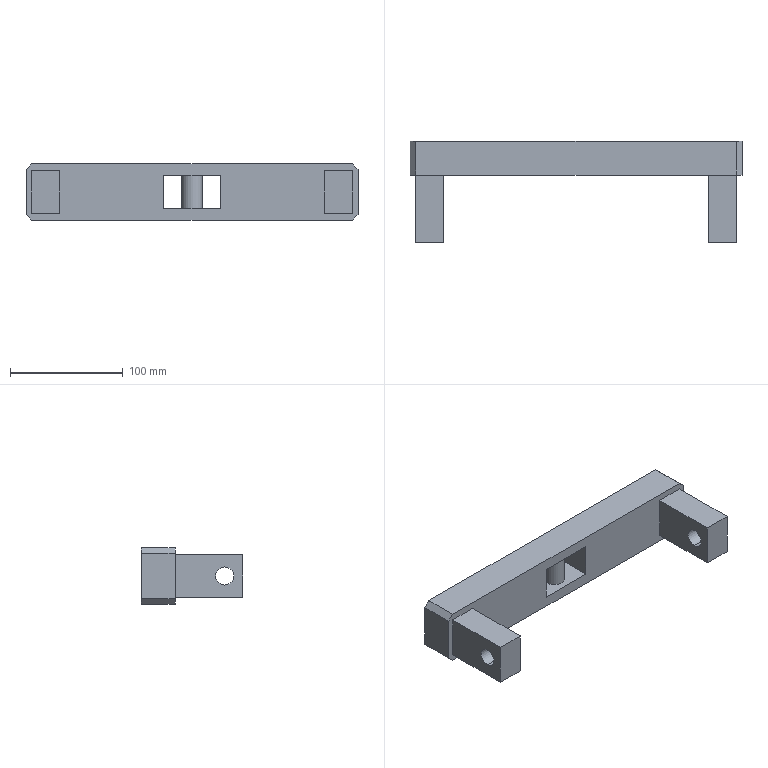Part | STEP file | PN_0003 Connecting bracket | 1 solid | 40 faces | box 295 x 90.05 x 50 mm | volume 507676 mm3 | plane 34 | cylinder 6 | commonest cylinder face diameters 16 x4 18 x2